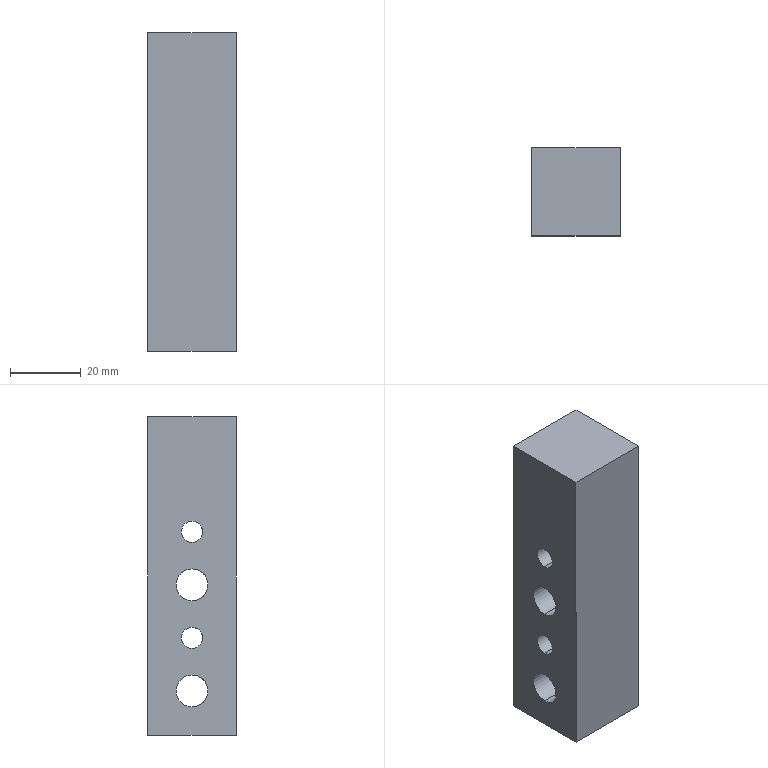Part | STEP file | Positioning_id1942_x_t | 1 solid | 20 faces | box 25 x 25 x 90 mm | volume 49849 mm3 | cylinder 12 | plane 8 | commonest cylinder face diameters 6 x4 9 x4 14 x4